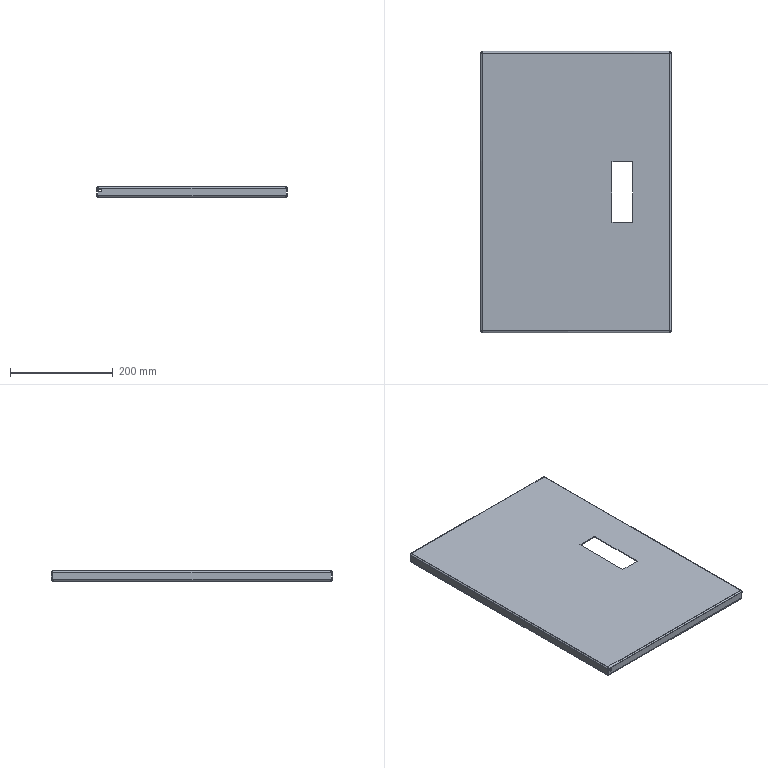Part | SolidWorks | features EdgeFlange 2, ICE 2, FlatPattern 1, SMBaseFlange 1, SheetMetal 1 | 1 solid | 78 faces | box 371 x 547 x 20 mm | volume 376908 mm3 | plane 42 | cylinder 20 | spline 16 | commonest cylinder face diameters 4 x8 7 x8 6 x4